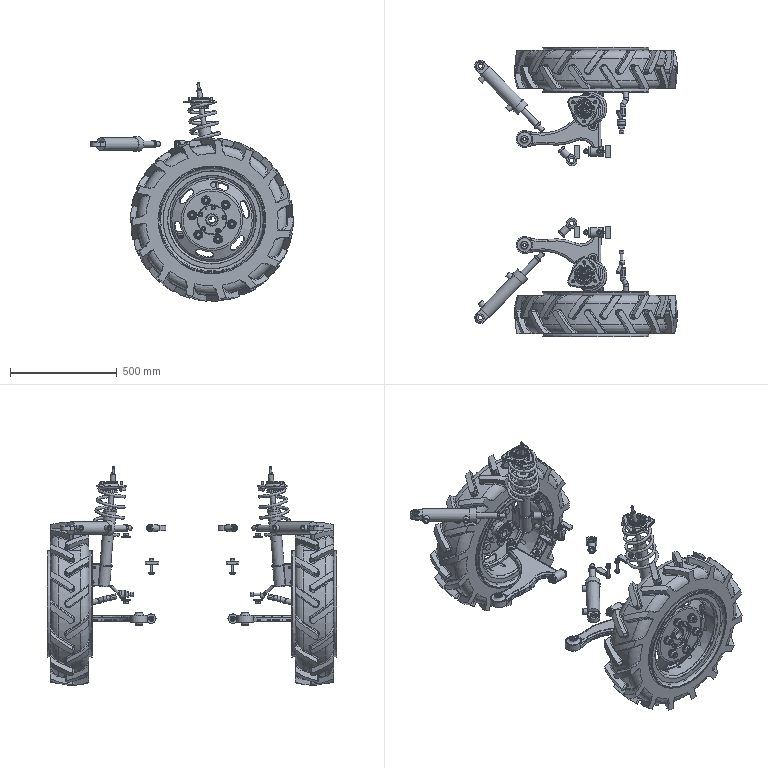Part | STEP file | COMPOUND | 233 solids | 4533 faces | volume 107297601 mm3 | plane 1928 | cylinder 1034 | cone 744 | spline 542 | torus 278 | sphere 7 | commonest cylinder face diameters 20 x152 84 x84 89 x84 16 x66 10 x42 12 x38